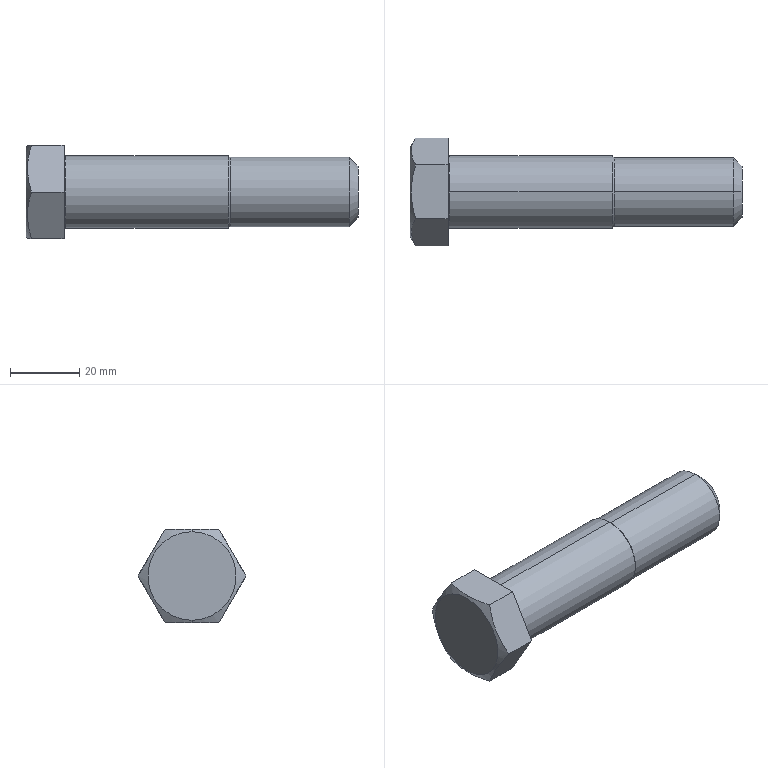Part | STEP file | Bolt M20x85 | 1 solid | 21 faces | box 96 x 31.2 x 27.02 mm | volume 34962 mm3 | plane 9 | cone 6 | cylinder 4 | torus 2 | commonest cylinder face diameters 20 x2 21 x2